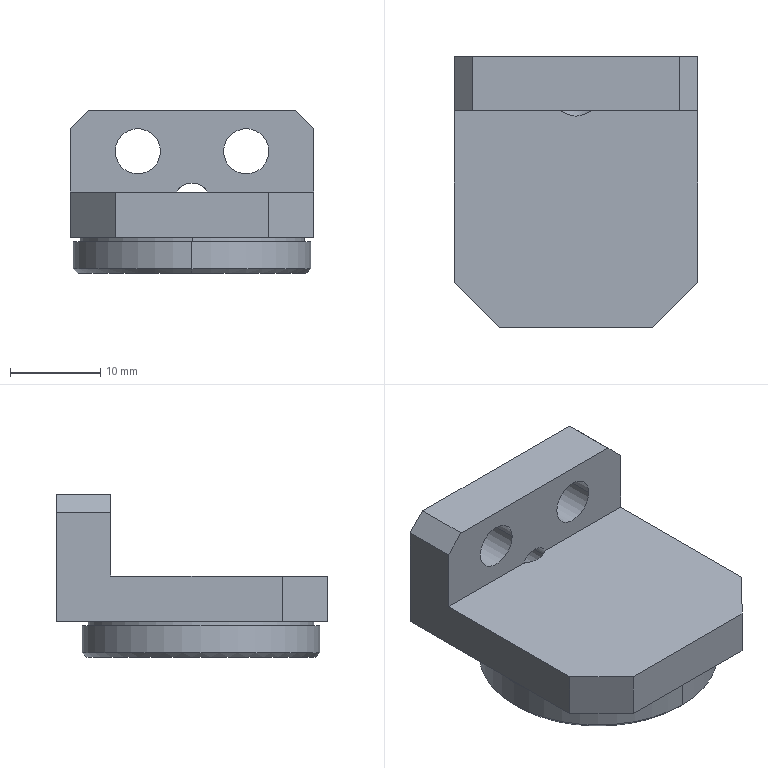NC program | NX | posted with a generic post | part box 27 x 30 x 18 mm
Whole program:
N10 G17 G21 G94 G90
(DRILLING , TOOL : D6A45)
N12 T07 M6
N14 G54
N16 G17 G0 G90 X0. Y10. B0. C0. S5000 M3
N18 G43 Z30. H7
N20 G94 G81 G98 Z-1. F250. R3.
N22 X-6. Y4.5
N24 X6.
N26 G80
N28 G0 X6. Y4.5 Z30.
N30 M5
(DRILLING_COPY , TOOL : 5.0ZT)
N32 T15 M6
N34 G54
N36 G17 G0 G90 X-6. Y4.5 B0. C0. S5000 M3
N38 G43 Z30. H15
N40 G94 G83 G98 Z-9.002 F250. Q2. R3.
N42 X6.
N44 G80
N46 G0 X6. Y4.5 Z30.
N48 M5
(ZLEVEL_PROFILE_COPY_COPY_1 , TOOL : D3)
N50 T03 M6
N52 G54
N54 G17 G0 G90 X-0.088 Y10.392 B0. C0. S9500 M3
N56 G43 Z30. H3
N58 Z1.
N60 G94 G1 X-0.209 Y10.353 Z0.993 F1000.
N62 X-0.331 Y10.242 Z0.985
N64 X-0.399 Y10.093 Z0.976
N66 X-0.401 Y9.913 Z0.967
N68 X-0.333 Y9.76 Z0.958
N70 X-0.209 Y9.647 Z0.949
N72 X-0.038 Y9.592 Z0.94
N74 X0.156 Y9.621 Z0.929
N76 X0.314 Y9.737 Z0.919
N78 X0.401 Y9.913 Z0.909
N80 X0.399 Y10.093 Z0.899
N82 X0.289 Y10.291 Z0.888
N84 X0.09 Y10.4 Z0.876
N86 X-0.063 Z0.868
N88 X-0.209 Y10.353 Z0.86
N90 X-0.331 Y10.242 Z0.851
N92 X-0.399 Y10.093 Z0.842
N94 X-0.401 Y9.913 Z0.833
N96 X-0.333 Y9.76 Z0.824
N98 X-0.209 Y9.647 Z0.815
N100 X-0.038 Y9.592 Z0.806
N102 X0.156 Y9.621 Z0.796
N104 X0.314 Y9.737 Z0.785
N106 X0.401 Y9.913 Z0.775
N108 X0.399 Y10.093 Z0.766
N110 X0.289 Y10.291 Z0.754
N112 X0.09 Y10.4 Z0.742
N114 X-0.063 Z0.734
N116 X-0.209 Y10.353 Z0.726
N118 X-0.331 Y10.242 Z0.717
N120 X-0.399 Y10.093 Z0.709
N122 X-0.401 Y9.913 Z0.699
N124 X-0.333 Y9.76 Z0.69
N126 X-0.209 Y9.647 Z0.682
N128 X-0.038 Y9.592 Z0.672
N130 X0.156 Y9.621 Z0.662
N132 X0.314 Y9.737 Z0.652
N134 X0.401 Y9.913 Z0.641
N136 X0.399 Y10.093 Z0.632
N138 X0.289 Y10.291 Z0.62
N140 X0.09 Y10.4 Z0.608
N142 X-0.063 Z0.6
N144 X-0.209 Y10.353 Z0.592
N146 X-0.331 Y10.242 Z0.583
N148 X-0.399 Y10.093 Z0.575
N150 X-0.401 Y9.913 Z0.565
N152 X-0.333 Y9.76 Z0.557
N154 X-0.209 Y9.647 Z0.548
N156 X-0.038 Y9.592 Z0.539
N158 X0.156 Y9.621 Z0.528
N160 X0.314 Y9.737 Z0.518
N162 X0.401 Y9.913 Z0.508
N164 X0.399 Y10.093 Z0.498
N166 X0.289 Y10.291 Z0.486
N168 X0.09 Y10.4 Z0.474
N170 X-0.063 Z0.466
N172 X-0.209 Y10.353 Z0.458
N174 X-0.331 Y10.242 Z0.45
N176 X-0.399 Y10.093 Z0.441
N178 X-0.401 Y9.913 Z0.432
N180 X-0.333 Y9.76 Z0.423
N182 X-0.209 Y9.647 Z0.414
N184 X-0.038 Y9.592 Z0.405
N186 X0.156 Y9.621 Z0.394
N188 X0.314 Y9.737 Z0.384
N190 X0.401 Y9.913 Z0.374
N192 X0.399 Y10.093 Z0.365
N194 X0.289 Y10.291 Z0.353
N196 X0.09 Y10.4 Z0.341
N198 X-0.063 Z0.333
N200 X-0.209 Y10.353 Z0.325
N202 X-0.331 Y10.242 Z0.316
N204 X-0.399 Y10.093 Z0.307
N206 X-0.401 Y9.913 Z0.298
N208 X-0.333 Y9.76 Z0.289
N210 X-0.209 Y9.647 Z0.28
N212 X-0.038 Y9.592 Z0.271
N214 X0.156 Y9.621 Z0.261
N216 X0.314 Y9.737 Z0.25
N218 X0.401 Y9.913 Z0.24
N220 X0.399 Y10.093 Z0.231
N222 X0.289 Y10.291 Z0.219
N224 X0.09 Y10.4 Z0.207
N226 X-0.063 Z0.199
N228 X-0.209 Y10.353 Z0.191
N230 X-0.331 Y10.242 Z0.182
N232 X-0.399 Y10.093 Z0.174
N234 X-0.401 Y9.913 Z0.164
N236 X-0.333 Y9.76 Z0.156
N238 X-0.209 Y9.647 Z0.147
N240 X-0.038 Y9.592 Z0.137
N242 X0.156 Y9.621 Z0.127
N244 X0.314 Y9.737 Z0.117
N246 X0.401 Y9.913 Z0.106
N248 X0.399 Y10.093 Z0.097
N250 X0.289 Y10.291 Z0.085
N252 X0.09 Y10.4 Z0.073
N254 X-0.063 Z0.065
N256 X-0.209 Y10.353 Z0.057
N258 X-0.331 Y10.242 Z0.049
N260 X-0.399 Y10.093 Z0.04
N262 X-0.401 Y9.913 Z0.031
N264 X-0.333 Y9.76 Z0.022
N266 X-0.209 Y9.647 Z0.013
N268 X-0.038 Y9.592 Z0.004
N270 X0.156 Y9.621 Z-0.007
N272 X0.314 Y9.737 Z-0.017
N274 X0.401 Y9.913 Z-0.027
N276 X0.399 Y10.093 Z-0.037
N278 X0.289 Y10.291 Z-0.049
N280 X0.09 Y10.4 Z-0.06
N282 X-0.063 Z-0.069
N284 X-0.209 Y10.353 Z-0.077
N286 X-0.331 Y10.242 Z-0.085
N288 X-0.399 Y10.093 Z-0.094
N290 X-0.401 Y9.913 Z-0.103
N292 X-0.333 Y9.76 Z-0.112
N294 X-0.209 Y9.647 Z-0.121
N296 X-0.038 Y9.592 Z-0.13
N298 X0.156 Y9.621 Z-0.14
N300 X0.314 Y9.737 Z-0.151
N302 X0.401 Y9.913 Z-0.161
N304 X0.399 Y10.093 Z-0.17
N306 X0.289 Y10.291 Z-0.182
N308 X0.09 Y10.4 Z-0.194
N310 X0. Z-0.199
N312 G3 X-0.4 Y10. R0.4 F1200.
N314 X0. Y10.4 R-0.4
N316 G1 X-0.095 Y10.379 Z-0.209
N318 X-0.141 Y10.365 Z-0.214
N320 X-0.167 Y10.354 Z-0.218
N322 X-0.218 Y10.326 Z-0.224
N324 X-0.288 Y10.265 Z-0.234
N326 X-0.317 Y10.23 Z-0.239
N328 X-0.334 Y10.204 Z-0.242
N330 X-0.362 Y10.15 Z-0.249
N332 X-0.387 Y10.06 Z-0.259
N334 X-0.391 Y10.014 Z-0.264
N336 Y9.984 Z-0.267
N338 X-0.385 Y9.924 Z-0.274
N340 X-0.355 Y9.835 Z-0.283
N342 X-0.333 Y9.795 Z-0.288
N344 X-0.316 Y9.77 Z-0.292
N346 X-0.277 Y9.723 Z-0.298
N348 X-0.203 Y9.666 Z-0.308
N350 X-0.163 Y9.644 Z-0.313
N352 X-0.135 Y9.633 Z-0.317
N354 X-0.076 Y9.616 Z-0.323
N356 X0.017 Y9.609 Z-0.333
N358 X0.062 Y9.614 Z-0.338
N360 X0.092 Y9.62 Z-0.341
N362 X0.15 Y9.638 Z-0.348
N364 X0.229 Y9.683 Z-0.358
N366 X0.287 Y9.732 Z-0.366
N368 X0.326 Y9.782 Z-0.373
N370 X0.354 Y9.834 Z-0.379
N372 X0.374 Y9.888 Z-0.385
N374 X0.387 Y9.944 Z-0.392
N376 X0.4 Y10. Z-0.398
N378 Y10.003
N380 G3 X0. Y10.4 R0.4
N382 G1 X-0.095 Y10.379 Z-0.408
N384 X-0.141 Y10.365 Z-0.413
N386 X-0.167 Y10.354 Z-0.416
N388 X-0.218 Y10.326 Z-0.423
N390 X-0.288 Y10.265 Z-0.433
N392 X-0.317 Y10.23 Z-0.438
N394 X-0.334 Y10.204 Z-0.441
N396 X-0.362 Y10.15 Z-0.448
N398 X-0.387 Y10.06 Z-0.457
N400 X-0.391 Y10.014 Z-0.462
N402 Y9.984 Z-0.466
N404 X-0.384 Y9.924 Z-0.472
N406 X-0.355 Y9.835 Z-0.482
N408 X-0.333 Y9.795 Z-0.487
N410 X-0.316 Y9.77 Z-0.491
N412 X-0.277 Y9.723 Z-0.497
N414 X-0.203 Y9.666 Z-0.507
N416 X-0.163 Y9.645 Z-0.512
N418 X-0.135 Y9.633 Z-0.516
N420 X-0.076 Y9.616 Z-0.522
N422 X0.017 Y9.61 Z-0.532
N424 X0.062 Y9.614 Z-0.537
N426 X0.092 Y9.62 Z-0.54
N428 X0.15 Y9.638 Z-0.547
N430 X0.229 Y9.683 Z-0.557
N432 X0.287 Y9.732 Z-0.565
N434 X0.326 Y9.782 Z-0.572
N436 X0.354 Y9.834 Z-0.578
N438 X0.374 Y9.888 Z-0.584
N440 X0.387 Y9.944 Z-0.591
N442 X0.4 Y10. Z-0.597
N444 Y10.003
N446 G3 X0. Y10.4 R0.4
N448 G1 X-0.095 Y10.379 Z-0.607
N450 X-0.141 Y10.365 Z-0.612
N452 X-0.167 Y10.354 Z-0.615
N454 X-0.218 Y10.326 Z-0.622
N456 X-0.288 Y10.265 Z-0.632
N458 X-0.317 Y10.23 Z-0.636
N460 X-0.334 Y10.204 Z-0.64
N462 X-0.362 Y10.15 Z-0.646
N464 X-0.387 Y10.06 Z-0.656
N466 X-0.391 Y10.014 Z-0.661
N468 Y9.984 Z-0.665
N470 X-0.384 Y9.924 Z-0.671
N472 X-0.355 Y9.835 Z-0.681
N474 X-0.333 Y9.795 Z-0.686
N476 X-0.316 Y9.77 Z-0.69
N478 X-0.277 Y9.723 Z-0.696
N480 X-0.203 Y9.666 Z-0.706
N482 X-0.163 Y9.645 Z-0.711
N484 X-0.135 Y9.633 Z-0.714
N486 X-0.076 Y9.616 Z-0.721
N488 X0.017 Y9.61 Z-0.731
N490 X0.062 Y9.614 Z-0.736
N492 X0.092 Y9.62 Z-0.739
N494 X0.15 Y9.638 Z-0.746
N496 X0.229 Y9.683 Z-0.756
N498 X0.287 Y9.732 Z-0.764
N500 X0.326 Y9.782 Z-0.771
N502 X0.354 Y9.834 Z-0.777
N504 X0.374 Y9.888 Z-0.783
N506 X0.387 Y9.944 Z-0.789
N508 X0.4 Y10. Z-0.796
N510 Y10.003
N512 G3 X0. Y10.4 R0.4
N514 G1 X-0.095 Y10.379 Z-0.806
N516 X-0.141 Y10.365 Z-0.811
N518 X-0.167 Y10.354 Z-0.814
N520 X-0.218 Y10.326 Z-0.821
N522 X-0.288 Y10.265 Z-0.83
N524 X-0.317 Y10.23 Z-0.835
N526 X-0.334 Y10.204 Z-0.839
N528 X-0.362 Y10.15 Z-0.845
N530 X-0.387 Y10.06 Z-0.855
N532 X-0.391 Y10.014 Z-0.86
N534 Y9.984 Z-0.864
N536 X-0.384 Y9.924 Z-0.87
N538 X-0.355 Y9.835 Z-0.88
N540 X-0.333 Y9.795 Z-0.885
N542 X-0.316 Y9.77 Z-0.888
N544 X-0.277 Y9.723 Z-0.895
N546 X-0.203 Y9.666 Z-0.905
N548 X-0.163 Y9.645 Z-0.91
N550 X-0.135 Y9.633 Z-0.913
N552 X-0.076 Y9.616 Z-0.92
N554 X0.017 Y9.61 Z-0.93
N556 X0.062 Y9.614 Z-0.935
N558 X0.092 Y9.62 Z-0.938
N560 X0.15 Y9.638 Z-0.945
N562 X0.229 Y9.683 Z-0.955
N564 X0.287 Y9.732 Z-0.963
N566 X0.326 Y9.782 Z-0.97
N568 X0.354 Y9.834 Z-0.976
N570 X0.374 Y9.888 Z-0.982
N572 X0.387 Y9.944 Z-0.988
N574 X0.4 Y10. Z-0.995
N576 Y10.003
N578 G3 X0. Y10.4 R0.4
N580 G1 X-0.095 Y10.379 Z-1.005
N582 X-0.141 Y10.365 Z-1.01
N584 X-0.167 Y10.354 Z-1.013
N586 X-0.218 Y10.326 Z-1.019
N588 X-0.288 Y10.265 Z-1.029
N590 X-0.317 Y10.23 Z-1.034
N592 X-0.334 Y10.204 Z-1.038
N594 X-0.362 Y10.15 Z-1.044
N596 X-0.387 Y10.06 Z-1.054
N598 X-0.391 Y10.014 Z-1.059
N600 Y9.984 Z-1.063
N602 X-0.384 Y9.924 Z-1.069
N604 X-0.354 Y9.835 Z-1.079
N606 X-0.333 Y9.795 Z-1.084
N608 X-0.316 Y9.77 Z-1.087
N610 X-0.277 Y9.723 Z-1.094
N612 X-0.203 Y9.666 Z-1.104
N614 X-0.163 Y9.645 Z-1.109
N616 X-0.135 Y9.633 Z-1.112
N618 X-0.076 Y9.616 Z-1.119
N620 X0.017 Y9.61 Z-1.129
N622 X0.062 Y9.614 Z-1.134
N624 X0.092 Y9.62 Z-1.137
N626 X0.15 Y9.638 Z-1.144
N628 X0.229 Y9.683 Z-1.153
N630 X0.286 Y9.732 Z-1.162
N632 X0.326 Y9.782 Z-1.169
N634 X0.354 Y9.834 Z-1.175
N636 X0.374 Y9.888 Z-1.181
N638 X0.387 Y9.944 Z-1.187
N640 X0.4 Y10. Z-1.194
N642 Y10.003
N644 G3 X0. Y10.4 R0.4
N646 G1 X-0.095 Y10.379 Z-1.204
N648 X-0.141 Y10.365 Z-1.209
N650 X-0.167 Y10.354 Z-1.212
N652 X-0.218 Y10.326 Z-1.218
N654 X-0.288 Y10.265 Z-1.228
N656 X-0.317 Y10.23 Z-1.233
N658 X-0.334 Y10.204 Z-1.237
N660 X-0.362 Y10.15 Z-1.243
N662 X-0.386 Y10.06 Z-1.253
N664 X-0.391 Y10.014 Z-1.258
N666 Y9.984 Z-1.261
N668 X-0.384 Y9.924 Z-1.268
N670 X-0.354 Y9.835 Z-1.278
N672 X-0.333 Y9.795 Z-1.283
N674 X-0.316 Y9.77 Z-1.286
N676 X-0.277 Y9.723 Z-1.293
N678 X-0.203 Y9.666 Z-1.303
N680 X-0.163 Y9.645 Z-1.308
N682 X-0.135 Y9.633 Z-1.311
N684 X-0.076 Y9.616 Z-1.318
N686 X0.016 Y9.61 Z-1.328
N688 X0.062 Y9.614 Z-1.333
N690 X0.091 Y9.62 Z-1.336
N692 X0.15 Y9.638 Z-1.343
N694 X0.229 Y9.683 Z-1.352
N696 X0.286 Y9.732 Z-1.361
N698 X0.326 Y9.782 Z-1.368
N700 X0.354 Y9.834 Z-1.374
N702 X0.374 Y9.888 Z-1.38
N704 X0.387 Y9.944 Z-1.386
N706 X0.4 Y10. Z-1.392
N708 Y10.003
N710 G3 X0. Y10.4 R0.4
N712 G1 X-0.095 Y10.379 Z-1.403
N714 X-0.141 Y10.365 Z-1.408
N716 X-0.167 Y10.353 Z-1.411
N718 X-0.218 Y10.326 Z-1.417
N720 X-0.288 Y10.265 Z-1.427
N722 X-0.317 Y10.23 Z-1.432
N724 X-0.334 Y10.204 Z-1.435
N726 X-0.362 Y10.15 Z-1.442
N728 X-0.386 Y10.06 Z-1.452
N730 X-0.391 Y10.014 Z-1.457
N732 Y9.984 Z-1.46
N734 X-0.384 Y9.924 Z-1.467
N736 X-0.354 Y9.835 Z-1.477
N738 X-0.333 Y9.796 Z-1.482
N740 X-0.316 Y9.77 Z-1.485
N742 X-0.277 Y9.723 Z-1.492
N744 X-0.203 Y9.667 Z-1.502
N746 X-0.163 Y9.645 Z-1.507
N748 X-0.135 Y9.633 Z-1.51
N750 X-0.076 Y9.616 Z-1.517
N752 X0.016 Y9.61 Z-1.527
N754 X0.061 Y9.614 Z-1.532
N756 X0.091 Y9.62 Z-1.535
N758 X0.15 Y9.638 Z-1.542
N760 X0.228 Y9.683 Z-1.551
N762 X0.264 Y9.71 Z-1.556
N764 X0.286 Y9.732 Z-1.56
N766 X0.326 Y9.782 Z-1.566
N768 X0.354 Y9.834 Z-1.573
N770 X0.374 Y9.888 Z-1.579
N772 X0.387 Y9.944 Z-1.585
N774 X0.4 Y10. Z-1.591
N776 Y10.003
N778 G3 X0. Y10.4 R0.4
N780 G1 X-0.095 Y10.379 Z-1.602
N782 X-0.14 Y10.365 Z-1.607
N784 X-0.167 Y10.353 Z-1.61
N786 X-0.218 Y10.326 Z-1.616
N788 X-0.288 Y10.265 Z-1.626
N790 X-0.317 Y10.23 Z-1.631
N792 X-0.334 Y10.204 Z-1.634
N794 X-0.362 Y10.15 Z-1.641
N796 X-0.386 Y10.06 Z-1.651
N798 X-0.391 Y10.015 Z-1.656
N800 Y9.984 Z-1.659
N802 X-0.384 Y9.924 Z-1.666
N804 X-0.354 Y9.835 Z-1.676
N806 X-0.333 Y9.796 Z-1.681
N808 X-0.316 Y9.77 Z-1.684
N810 X-0.277 Y9.723 Z-1.691
N812 X-0.204 Y9.665 Z-1.701
N814 X-0.164 Y9.644 Z-1.706
N816 X-0.135 Y9.634 Z-1.709
N818 X-0.076 Y9.616 Z-1.716
N820 X0.016 Y9.61 Z-1.726
N822 X0.061 Y9.614 Z-1.73
N824 X0.091 Y9.62 Z-1.734
N826 X0.15 Y9.638 Z-1.741
N828 X0.23 Y9.682 Z-1.75
N830 X0.264 Y9.71 Z-1.755
N832 X0.286 Y9.732 Z-1.758
N834 X0.325 Y9.783 Z-1.765
N836 X0.354 Y9.834 Z-1.772
N838 X0.374 Y9.888 Z-1.778
N840 X0.387 Y9.944 Z-1.784
N842 X0.4 Y10. Z-1.79
N844 Y10.003
N846 G3 X0. Y10.4 R0.4
N848 G1 X-0.095 Y10.379 Z-1.801
N850 X-0.14 Y10.365 Z-1.806
N852 X-0.167 Y10.353 Z-1.809
N854 X-0.218 Y10.326 Z-1.815
N856 X-0.288 Y10.265 Z-1.825
N858 X-0.316 Y10.23 Z-1.83
N860 X-0.334 Y10.204 Z-1.833
N862 X-0.362 Y10.15 Z-1.84
N864 X-0.386 Y10.06 Z-1.85
N866 X-0.391 Y10.015 Z-1.855
N868 Y9.984 Z-1.858
N870 X-0.384 Y9.924 Z-1.865
N872 X-0.354 Y9.835 Z-1.875
N874 X-0.333 Y9.796 Z-1.88
N876 X-0.316 Y9.77 Z-1.883
N878 X-0.277 Y9.723 Z-1.89
N880 X-0.204 Y9.665 Z-1.9
N882 X-0.164 Y9.644 Z-1.905
N884 X-0.135 Y9.634 Z-1.908
N886 X-0.076 Y9.616 Z-1.915
N888 X0.017 Y9.608 Z-1.924
N890 X0.061 Y9.613 Z-1.929
N892 X0.091 Y9.62 Z-1.933
N894 X0.15 Y9.638 Z-1.939
N896 X0.229 Y9.682 Z-1.949
N898 X0.263 Y9.71 Z-1.954
N900 X0.286 Y9.732 Z-1.957
N902 X0.325 Y9.783 Z-1.964
N904 X0.354 Y9.834 Z-1.971
N906 X0.374 Y9.888 Z-1.977
N908 X0.387 Y9.944 Z-1.983
N910 X0.4 Y10. Z-1.989
N912 Y10.003
N914 G3 X0. Y10.4 R0.4
N916 G1 X-0.095 Y10.379 Z-1.999
N918 X-0.14 Y10.365 Z-2.005
N920 X-0.167 Y10.353 Z-2.008
N922 X-0.218 Y10.326 Z-2.014
N924 X-0.288 Y10.265 Z-2.024
N926 X-0.316 Y10.23 Z-2.029
N928 X-0.333 Y10.204 Z-2.032
N930 X-0.362 Y10.15 Z-2.039
N932 X-0.386 Y10.06 Z-2.049
N934 X-0.391 Y10.015 Z-2.054
N936 Y9.984 Z-2.057
N938 X-0.384 Y9.924 Z-2.064
N940 X-0.354 Y9.836 Z-2.074
N942 X-0.333 Y9.796 Z-2.079
N944 X-0.316 Y9.77 Z-2.082
N946 X-0.277 Y9.723 Z-2.089
N948 X-0.204 Y9.665 Z-2.099
N950 X-0.164 Y9.644 Z-2.103
N952 X-0.136 Y9.632 Z-2.107
N954 X-0.076 Y9.616 Z-2.114
N956 X0.019 Y9.609 Z-2.124
N958 X0.065 Y9.613 Z-2.129
N960 X0.15 Y9.638 Z-2.138
N962 X0.23 Y9.682 Z-2.148
N964 X0.264 Y9.711 Z-2.153
N966 X0.286 Y9.733 Z-2.156
N968 X0.325 Y9.783 Z-2.163
N970 X0.354 Y9.834 Z-2.169
N972 X0.374 Y9.888 Z-2.176
N974 X0.387 Y9.944 Z-2.182
N976 X0.4 Y10. Z-2.188
N978 Y10.003
N980 G3 X0. Y10.4 R0.4
N982 G1 X-0.095 Y10.379 Z-2.198
N984 X-0.14 Y10.365 Z-2.204
N986 X-0.167 Y10.353 Z-2.207
N988 X-0.218 Y10.326 Z-2.213
N990 X-0.288 Y10.265 Z-2.223
N992 X-0.316 Y10.23 Z-2.228
N994 X-0.333 Y10.204 Z-2.231
N996 X-0.362 Y10.15 Z-2.238
N998 X-0.386 Y10.06 Z-2.248
N1000 X-0.391 Y10.015 Z-2.253
N1002 Y9.984 Z-2.256
N1004 X-0.384 Y9.924 Z-2.263
N1006 X-0.354 Y9.836 Z-2.273
N1008 X-0.333 Y9.796 Z-2.278
N1010 X-0.316 Y9.771 Z-2.281
N1012 X-0.277 Y9.723 Z-2.288
N1014 X-0.204 Y9.665 Z-2.297
N1016 X-0.164 Y9.644 Z-2.302
N1018 X-0.136 Y9.632 Z-2.306
N1020 X-0.076 Y9.616 Z-2.312
N1022 X0.019 Y9.609 Z-2.323
N1024 X0.065 Y9.613 Z-2.328
N1026 X0.15 Y9.638 Z-2.337
N1028 X0.229 Y9.682 Z-2.347
N1030 X0.264 Y9.71 Z-2.352
N1032 X0.286 Y9.733 Z-2.355
N1034 X0.325 Y9.783 Z-2.362
N1036 X0.354 Y9.834 Z-2.368
N1038 X0.374 Y9.888 Z-2.375
N1040 X0.387 Y9.944 Z-2.381
N1042 X0.4 Y10. Z-2.387
N1044 Y10.003
N1046 G3 X0. Y10.4 R0.4
N1048 G1 X-0.094 Y10.379 Z-2.397
N1050 X-0.14 Y10.365 Z-2.402
N1052 X-0.167 Y10.353 Z-2.406
N1054 X-0.218 Y10.326 Z-2.412
N1056 X-0.288 Y10.265 Z-2.422
N1058 X-0.316 Y10.23 Z-2.427
N1060 X-0.333 Y10.204 Z-2.43
N1062 X-0.362 Y10.15 Z-2.437
N1064 X-0.386 Y10.06 Z-2.447
N1066 X-0.391 Y10.015 Z-2.452
N1068 Y9.984 Z-2.455
N1070 X-0.384 Y9.924 Z-2.462
N1072 X-0.354 Y9.836 Z-2.471
N1074 X-0.317 Y9.77 Z-2.48
N1076 X-0.277 Y9.723 Z-2.486
N1078 X-0.201 Y9.664 Z-2.497
N1080 X-0.161 Y9.643 Z-2.502
N1082 X-0.076 Y9.616 Z-2.511
N1084 X0.017 Y9.609 Z-2.521
N1086 X0.062 Y9.613 Z-2.526
N1088 X0.092 Y9.619 Z-2.53
N1090 X0.15 Y9.638 Z-2.536
N1092 X0.231 Y9.684 Z-2.546
N1094 X0.266 Y9.713 Z-2.551
N1096 X0.287 Y9.734 Z-2.554
N1098 X0.325 Y9.783 Z-2.561
N1100 X0.354 Y9.834 Z-2.567
N1102 X0.374 Y9.888 Z-2.574
N1104 X0.387 Y9.944 Z-2.58
N1106 X0.4 Y10. Z-2.586
N1108 Y10.003
N1110 G3 X0. Y10.4 R0.4
N1112 G1 X-0.094 Y10.379 Z-2.596
N1114 X-0.14 Y10.365 Z-2.601
N1116 X-0.167 Y10.353 Z-2.605
N1118 X-0.218 Y10.326 Z-2.611
N1120 X-0.288 Y10.265 Z-2.621
N1122 X-0.316 Y10.23 Z-2.626
N1124 X-0.333 Y10.204 Z-2.629
N1126 X-0.362 Y10.15 Z-2.636
N1128 X-0.386 Y10.06 Z-2.646
N1130 X-0.391 Y10.015 Z-2.651
N1132 Y9.984 Z-2.654
N1134 X-0.384 Y9.924 Z-2.661
N1136 X-0.354 Y9.836 Z-2.67
N1138 X-0.334 Y9.795 Z-2.675
N1140 X-0.317 Y9.77 Z-2.679
N1142 X-0.277 Y9.723 Z-2.685
N1144 X-0.201 Y9.665 Z-2.695
N1146 X-0.161 Y9.643 Z-2.701
N1148 X-0.076 Y9.616 Z-2.71
N1150 X0.017 Y9.609 Z-2.72
N1152 X0.062 Y9.613 Z-2.725
N1154 X0.091 Y9.619 Z-2.728
N1156 X0.15 Y9.639 Z-2.735
N1158 X0.231 Y9.684 Z-2.745
N1160 X0.266 Y9.713 Z-2.75
N1162 X0.287 Y9.734 Z-2.753
N1164 X0.325 Y9.783 Z-2.76
N1166 X0.354 Y9.834 Z-2.766
N1168 X0.374 Y9.888 Z-2.772
N1170 X0.387 Y9.944 Z-2.779
N1172 X0.4 Y10. Z-2.785
N1174 Y10.003
N1176 G3 X0. Y10.4 R0.4
N1178 G1 X-0.094 Y10.379 Z-2.795
N1180 X-0.14 Y10.365 Z-2.8
N1182 X-0.167 Y10.353 Z-2.803
N1184 X-0.218 Y10.326 Z-2.81
N1186 X-0.288 Y10.265 Z-2.82
N1188 X-0.316 Y10.23 Z-2.825
N1190 X-0.333 Y10.204 Z-2.828
N1192 X-0.362 Y10.15 Z-2.835
N1194 X-0.386 Y10.06 Z-2.844
N1196 X-0.391 Y10.015 Z-2.849
N1198 Y9.984 Z-2.853
N1200 X-0.384 Y9.924 Z-2.859
N1202 X-0.354 Y9.836 Z-2.869
N1204 X-0.334 Y9.795 Z-2.874
N1206 X-0.317 Y9.77 Z-2.878
N1208 X-0.277 Y9.723 Z-2.884
N1210 X-0.202 Y9.665 Z-2.894
N1212 X-0.161 Y9.643 Z-2.899
N1214 X-0.076 Y9.616 Z-2.909
N1216 X0.017 Y9.609 Z-2.919
N1218 X0.061 Y9.613 Z-2.924
N1220 X0.091 Y9.619 Z-2.927
N1222 X0.15 Y9.639 Z-2.934
N1224 X0.231 Y9.684 Z-2.944
N1226 X0.265 Y9.712 Z-2.949
N1228 X0.287 Y9.734 Z-2.952
N1230 X0.325 Y9.783 Z-2.959
N1232 X0.354 Y9.834 Z-2.965
N1234 X0.374 Y9.888 Z-2.971
N1236 X0.387 Y9.944 Z-2.978
N1238 X0.4 Y10. Z-2.984
N1240 Y10.003
N1242 G3 X0. Y10.4 R0.4
N1244 G1 X-0.094 Y10.379 Z-2.994
N1246 X-0.14 Y10.365 Z-2.999
N1248 X-0.167 Y10.353 Z-3.002
N1250 X-0.218 Y10.326 Z-3.009
N1252 X-0.287 Y10.265 Z-3.018
N1254 X-0.316 Y10.23 Z-3.023
N1256 X-0.333 Y10.204 Z-3.027
N1258 X-0.362 Y10.15 Z-3.034
N1260 X-0.386 Y10.06 Z-3.043
N1262 X-0.39 Y10.015 Z-3.048
N1264 X-0.391 Y9.984 Z-3.052
N1266 X-0.384 Y9.924 Z-3.058
N1268 X-0.354 Y9.836 Z-3.068
N1270 X-0.334 Y9.796 Z-3.073
N1272 X-0.317 Y9.77 Z-3.077
N1274 X-0.277 Y9.723 Z-3.083
N1276 X-0.202 Y9.665 Z-3.093
N1278 X-0.161 Y9.643 Z-3.098
N1280 X-0.134 Y9.632 Z-3.102
N1282 X-0.076 Y9.616 Z-3.108
N1284 X0.019 Y9.609 Z-3.118
N1286 X0.065 Y9.614 Z-3.123
N1288 X0.15 Y9.639 Z-3.133
N1290 X0.229 Y9.683 Z-3.143
N1292 X0.263 Y9.71 Z-3.147
N1294 X0.285 Y9.733 Z-3.151
N1296 X0.325 Y9.783 Z-3.158
N1298 X0.354 Y9.834 Z-3.164
N1300 X0.374 Y9.888 Z-3.17
N1302 X0.387 Y9.944 Z-3.176
N1304 X0.4 Y10. Z-3.183
N1306 Y10.003
N1308 G3 X0. Y10.4 R0.4
N1310 G1 X-0.094 Y10.379 Z-3.193
N1312 X-0.14 Y10.365 Z-3.198
N1314 X-0.167 Y10.353 Z-3.201
N1316 X-0.218 Y10.326 Z-3.208
N1318 X-0.287 Y10.265 Z-3.217
N1320 X-0.316 Y10.23 Z-3.222
N1322 X-0.333 Y10.204 Z-3.226
N1324 X-0.362 Y10.15 Z-3.232
N1326 X-0.386 Y10.06 Z-3.242
N1328 X-0.39 Y10.015 Z-3.247
N1330 X-0.391 Y9.985 Z-3.251
N1332 X-0.384 Y9.924 Z-3.257
N1334 X-0.355 Y9.835 Z-3.267
N1336 X-0.334 Y9.796 Z-3.272
N1338 X-0.317 Y9.77 Z-3.275
N1340 X-0.277 Y9.723 Z-3.282
N1342 X-0.202 Y9.665 Z-3.292
N1344 X-0.161 Y9.643 Z-3.297
N1346 X-0.134 Y9.632 Z-3.301
N1348 X-0.076 Y9.616 Z-3.307
N1350 X0.019 Y9.609 Z-3.317
N1352 X0.065 Y9.614 Z-3.322
N1354 X0.094 Y9.62 Z-3.325
N1356 X0.15 Y9.639 Z-3.332
N1358 X0.231 Y9.684 Z-3.342
N1360 X0.266 Y9.713 Z-3.347
N1362 X0.287 Y9.735 Z-3.35
N1364 X0.325 Y9.783 Z-3.357
N1366 X0.354 Y9.834 Z-3.363
N1368 X0.374 Y9.888 Z-3.369
N1370 X0.387 Y9.944 Z-3.375
N1372 X0.4 Y10. Z-3.382
N1374 Y10.003
N1376 G3 X0. Y10.4 R0.4
N1378 G1 X-0.094 Y10.379 Z-3.392
N1380 X-0.14 Y10.365 Z-3.397
N1382 X-0.166 Y10.353 Z-3.4
N1384 X-0.218 Y10.326 Z-3.406
N1386 X-0.287 Y10.265 Z-3.416
N1388 X-0.316 Y10.23 Z-3.421
N1390 X-0.333 Y10.204 Z-3.425
N1392 X-0.362 Y10.15 Z-3.431
N1394 X-0.386 Y10.06 Z-3.441
N1396 X-0.39 Y10.015 Z-3.446
N1398 X-0.391 Y9.985 Z-3.45
N1400 X-0.384 Y9.924 Z-3.456
N1402 X-0.355 Y9.836 Z-3.466
N1404 X-0.334 Y9.796 Z-3.471
N1406 X-0.317 Y9.77 Z-3.474
N1408 X-0.277 Y9.723 Z-3.481
N1410 X-0.202 Y9.665 Z-3.491
N1412 X-0.161 Y9.643 Z-3.496
N1414 X-0.134 Y9.632 Z-3.499
N1416 X-0.076 Y9.616 Z-3.506
N1418 X0.019 Y9.61 Z-3.516
N1420 X0.065 Y9.614 Z-3.521
N1422 X0.094 Y9.62 Z-3.524
N1424 X0.15 Y9.639 Z-3.531
N1426 X0.231 Y9.684 Z-3.541
N1428 X0.266 Y9.713 Z-3.546
N1430 X0.287 Y9.735 Z-3.549
N1432 X0.325 Y9.783 Z-3.556
N1434 X0.354 Y9.834 Z-3.562
N1436 X0.374 Y9.888 Z-3.568
N1438 X0.387 Y9.944 Z-3.574
N1440 X0.4 Y10. Z-3.581
N1442 Y10.003
N1444 G3 X0. Y10.4 R0.4
N1446 G1 X-0.094 Y10.379 Z-3.591
N1448 X-0.14 Y10.365 Z-3.596
N1450 X-0.166 Y10.353 Z-3.599
N1452 X-0.218 Y10.326 Z-3.605
N1454 X-0.287 Y10.265 Z-3.615
N1456 X-0.316 Y10.23 Z-3.62
N1458 X-0.333 Y10.204 Z-3.624
N1460 X-0.362 Y10.15 Z-3.63
N1462 X-0.386 Y10.06 Z-3.64
N1464 X-0.39 Y10.015 Z-3.645
N1466 Y9.985 Z-3.648
N1468 X-0.384 Y9.924 Z-3.655
N1470 X-0.355 Y9.836 Z-3.665
N1472 X-0.334 Y9.796 Z-3.67
N1474 X-0.317 Y9.77 Z-3.673
N1476 X-0.276 Y9.724 Z-3.68
N1478 X-0.202 Y9.665 Z-3.69
N1480 X-0.161 Y9.643 Z-3.695
N1482 X-0.134 Y9.632 Z-3.698
N1484 X-0.076 Y9.617 Z-3.705
N1486 X0.019 Y9.61 Z-3.715
N1488 X0.065 Y9.614 Z-3.72
N1490 X0.093 Y9.62 Z-3.723
N1492 X0.15 Y9.639 Z-3.73
N1494 X0.231 Y9.684 Z-3.74
N1496 X0.265 Y9.713 Z-3.745
N1498 X0.287 Y9.735 Z-3.748
N1500 X0.325 Y9.783 Z-3.755
N1502 X0.354 Y9.834 Z-3.761
N1504 X0.374 Y9.888 Z-3.767
N1506 X0.387 Y9.944 Z-3.773
N1508 X0.4 Y10. Z-3.779
N1510 Y10.003
N1512 G3 X0. Y10.4 R0.4
N1514 G1 X-0.094 Y10.379 Z-3.79
N1516 X-0.14 Y10.365 Z-3.795
N1518 X-0.166 Y10.353 Z-3.798
N1520 X-0.218 Y10.326 Z-3.804
N1522 X-0.287 Y10.265 Z-3.814
N1524 X-0.316 Y10.23 Z-3.819
N1526 X-0.333 Y10.204 Z-3.822
N1528 X-0.362 Y10.15 Z-3.829
N1530 X-0.386 Y10.06 Z-3.839
N1532 X-0.39 Y10.015 Z-3.844
N1534 Y9.985 Z-3.847
N1536 X-0.384 Y9.924 Z-3.854
N1538 X-0.355 Y9.836 Z-3.864
N1540 X-0.334 Y9.796 Z-3.869
N1542 X-0.317 Y9.77 Z-3.872
N1544 X-0.276 Y9.724 Z-3.879
N1546 X-0.202 Y9.665 Z-3.889
N1548 X-0.161 Y9.644 Z-3.894
N1550 X-0.134 Y9.632 Z-3.897
N1552 X-0.076 Y9.617 Z-3.904
N1554 X0.019 Y9.61 Z-3.914
N1556 X0.064 Y9.614 Z-3.919
N1558 X0.093 Y9.62 Z-3.922
N1560 X0.15 Y9.639 Z-3.929
N1562 X0.23 Y9.684 Z-3.938
N1564 X0.265 Y9.713 Z-3.943
N1566 X0.287 Y9.735 Z-3.947
N1568 X0.325 Y9.783 Z-3.954
N1570 X0.354 Y9.834 Z-3.96
N1572 X0.374 Y9.888 Z-3.966
N1574 X0.387 Y9.944 Z-3.972
N1576 X0.4 Y10. Z-3.978
N1578 Y10.003
N1580 G3 X0. Y10.4 R0.4
N1582 G1 X-0.094 Y10.379 Z-3.989
N1584 X-0.14 Y10.365 Z-3.994
N1586 X-0.167 Y10.354 Z-3.997
N1588 X-0.218 Y10.326 Z-4.003
N1590 X-0.288 Y10.264 Z-4.013
N1592 X-0.317 Y10.228 Z-4.018
N1594 X-0.334 Y10.203 Z-4.021
N1596 X-0.362 Y10.15 Z-4.028
N1598 X-0.386 Y10.06 Z-4.038
N1600 X-0.39 Y10.015 Z-4.043
N1602 Y9.984 Z-4.046
N1604 X-0.384 Y9.924 Z-4.053
N1606 X-0.355 Y9.836 Z-4.063
N1608 X-0.334 Y9.796 Z-4.068
N1610 X-0.317 Y9.771 Z-4.071
N1612 X-0.276 Y9.724 Z-4.078
N1614 X-0.202 Y9.665 Z-4.088
N1616 X-0.161 Y9.644 Z-4.093
N1618 X-0.134 Y9.632 Z-4.096
N1620 X-0.076 Y9.617 Z-4.103
N1622 X0.018 Y9.61 Z-4.113
N1624 X0.064 Y9.614 Z-4.118
N1626 X0.093 Y9.62 Z-4.121
N1628 X0.15 Y9.639 Z-4.128
N1630 X0.23 Y9.684 Z-4.137
N1632 X0.265 Y9.713 Z-4.142
N1634 X0.287 Y9.735 Z-4.146
N1636 X0.325 Y9.783 Z-4.152
N1638 X0.354 Y9.834 Z-4.159
N1640 X0.374 Y9.888 Z-4.165
N1642 X0.387 Y9.944 Z-4.171
N1644 X0.4 Y10. Z-4.177
N1646 Y10.003
N1648 G3 X0. Y10.4 R0.4
N1650 G1 X-0.094 Y10.379 Z-4.188
N1652 X-0.14 Y10.365 Z-4.193
N1654 X-0.167 Y10.354 Z-4.196
N1656 X-0.218 Y10.326 Z-4.202
N1658 X-0.288 Y10.264 Z-4.212
N1660 X-0.317 Y10.228 Z-4.217
N1662 X-0.334 Y10.203 Z-4.22
N1664 X-0.362 Y10.15 Z-4.227
N1666 X-0.386 Y10.06 Z-4.237
N1668 X-0.39 Y10.015 Z-4.242
N1670 Y9.984 Z-4.245
N1672 X-0.384 Y9.924 Z-4.252
N1674 X-0.355 Y9.836 Z-4.262
N1676 X-0.334 Y9.796 Z-4.267
N1678 X-0.317 Y9.771 Z-4.27
N1680 X-0.276 Y9.724 Z-4.277
N1682 X-0.202 Y9.666 Z-4.287
N1684 X-0.161 Y9.644 Z-4.292
N1686 X-0.134 Y9.633 Z-4.295
N1688 X-0.076 Y9.617 Z-4.302
N1690 X0.018 Y9.61 Z-4.312
N1692 X0.064 Y9.614 Z-4.317
N1694 X0.093 Y9.62 Z-4.32
N1696 X0.15 Y9.639 Z-4.326
N1698 X0.23 Y9.684 Z-4.336
N1700 X0.265 Y9.713 Z-4.341
N1702 X0.286 Y9.735 Z-4.345
N1704 X0.325 Y9.783 Z-4.351
N1706 X0.354 Y9.834 Z-4.358
N1708 X0.374 Y9.888 Z-4.364
N1710 X0.387 Y9.944 Z-4.37
N1712 X0.4 Y10. Z-4.376
N1714 Y10.003
N1716 G3 X0. Y10.4 R0.4
N1718 G1 X-0.094 Y10.379 Z-4.386
N1720 X-0.14 Y10.365 Z-4.392
N1722 X-0.167 Y10.354 Z-4.395
N1724 X-0.218 Y10.326 Z-4.401
N1726 X-0.288 Y10.264 Z-4.411
N1728 X-0.317 Y10.228 Z-4.416
N1730 X-0.334 Y10.203 Z-4.419
N1732 X-0.362 Y10.15 Z-4.426
N1734 X-0.386 Y10.06 Z-4.436
N1736 X-0.39 Y10.015 Z-4.441
N1738 Y9.984 Z-4.444
N1740 X-0.384 Y9.924 Z-4.451
N1742 X-0.355 Y9.836 Z-4.461
N1744 X-0.334 Y9.796 Z-4.466
N1746 X-0.317 Y9.771 Z-4.469
N1748 X-0.276 Y9.724 Z-4.476
N1750 X-0.202 Y9.666 Z-4.486
N1752 X-0.161 Y9.644 Z-4.491
N1754 X-0.134 Y9.633 Z-4.494
N1756 X-0.076 Y9.617 Z-4.501
N1758 X0.018 Y9.61 Z-4.511
N1760 X0.064 Y9.614 Z-4.516
N1762 X0.093 Y9.62 Z-4.519
N1764 X0.15 Y9.639 Z-4.525
N1766 X0.23 Y9.684 Z-4.535
N1768 X0.265 Y9.713 Z-4.54
N1770 X0.286 Y9.735 Z-4.544
N1772 X0.325 Y9.783 Z-4.55
N1774 X0.354 Y9.834 Z-4.556
N1776 X0.374 Y9.888 Z-4.563
N1778 X0.387 Y9.944 Z-4.569
N1780 X0.4 Y10. Z-4.575
N1782 Y10.003
N1784 G3 X0. Y10.4 R0.4
N1786 G1 X-0.094 Y10.379 Z-4.585
N1788 X-0.14 Y10.365 Z-4.591
N1790 X-0.167 Y10.354 Z-4.594
N1792 X-0.218 Y10.326 Z-4.6
N1794 X-0.288 Y10.264 Z-4.61
N1796 X-0.317 Y10.228 Z-4.615
N1798 X-0.333 Y10.203 Z-4.618
N1800 X-0.362 Y10.15 Z-4.625
N1802 X-0.386 Y10.06 Z-4.635
N1804 X-0.39 Y10.015 Z-4.64
N1806 Y9.985 Z-4.643
N1808 X-0.384 Y9.924 Z-4.65
N1810 X-0.355 Y9.836 Z-4.66
N1812 X-0.334 Y9.796 Z-4.664
N1814 X-0.317 Y9.771 Z-4.668
N1816 X-0.276 Y9.724 Z-4.675
N1818 X-0.202 Y9.666 Z-4.685
N1820 X-0.161 Y9.644 Z-4.69
N1822 X-0.134 Y9.633 Z-4.693
N1824 X-0.076 Y9.617 Z-4.699
N1826 X0.018 Y9.61 Z-4.709
N1828 X0.064 Y9.614 Z-4.715
N1830 X0.093 Y9.62 Z-4.718
N1832 X0.15 Y9.639 Z-4.724
N1834 X0.23 Y9.684 Z-4.734
N1836 X0.264 Y9.713 Z-4.739
N1838 X0.286 Y9.734 Z-4.742
N1840 X0.325 Y9.783 Z-4.749
N1842 X0.354 Y9.834 Z-4.755
N1844 X0.374 Y9.888 Z-4.762
N1846 X0.387 Y9.944 Z-4.768
N1848 X0.4 Y10. Z-4.774
N1850 Y10.003
N1852 G3 X0. Y10.4 R0.4
N1854 G1 X-0.094 Y10.379 Z-4.784
N1856 X-0.14 Y10.365 Z-4.789
N1858 X-0.167 Y10.354 Z-4.793
N1860 X-0.218 Y10.326 Z-4.799
N1862 X-0.288 Y10.264 Z-4.809
N1864 X-0.317 Y10.229 Z-4.814
N1866 X-0.333 Y10.203 Z-4.817
N1868 X-0.362 Y10.15 Z-4.824
N1870 X-0.386 Y10.06 Z-4.834
N1872 X-0.39 Y10.015 Z-4.839
N1874 Y9.985 Z-4.842
N1876 X-0.384 Y9.924 Z-4.849
N1878 X-0.355 Y9.836 Z-4.858
N1880 X-0.334 Y9.797 Z-4.863
N1882 X-0.317 Y9.771 Z-4.867
N1884 X-0.276 Y9.724 Z-4.874
N1886 X-0.202 Y9.666 Z-4.884
N1888 X-0.161 Y9.644 Z-4.889
N1890 X-0.134 Y9.633 Z-4.892
N1892 X-0.076 Y9.617 Z-4.898
N1894 X0.018 Y9.61 Z-4.908
N1896 X0.064 Y9.615 Z-4.913
N1898 X0.093 Y9.62 Z-4.917
N1900 X0.15 Y9.639 Z-4.923
N1902 X0.23 Y9.684 Z-4.933
N1904 X0.264 Y9.713 Z-4.938
N1906 X0.286 Y9.734 Z-4.941
N1908 X0.325 Y9.783 Z-4.948
N1910 X0.354 Y9.834 Z-4.954
N1912 X0.374 Y9.888 Z-4.961
N1914 X0.386 Y9.944 Z-4.967
N1916 X0.4 Y10. Z-4.973
N1918 Y10.003
N1920 G3 X0. Y10.4 R0.4
N1922 G1 X-0.094 Y10.379 Z-4.983
N1924 X-0.14 Y10.365 Z-4.988
N1926 X-0.167 Y10.354 Z-4.992
N1928 X-0.218 Y10.326 Z-4.998
N1930 X-0.288 Y10.264 Z-5.008
N1932 X-0.317 Y10.229 Z-5.013
N1934 X-0.333 Y10.203 Z-5.016
N1936 X-0.362 Y10.15 Z-5.023
N1938 X-0.386 Y10.06 Z-5.033
N1940 X-0.39 Y10.015 Z-5.038
N1942 Y9.985 Z-5.041
N1944 X-0.384 Y9.924 Z-5.048
N1946 X-0.355 Y9.836 Z-5.057
N1948 X-0.334 Y9.797 Z-5.062
N1950 X-0.317 Y9.771 Z-5.066
N1952 X-0.276 Y9.724 Z-5.072
N1954 X-0.202 Y9.666 Z-5.082
N1956 X-0.162 Y9.644 Z-5.087
N1958 X-0.134 Y9.633 Z-5.091
N1960 X-0.076 Y9.617 Z-5.097
N1962 X0.018 Y9.61 Z-5.107
N1964 X0.063 Y9.615 Z-5.112
N1966 X0.093 Y9.621 Z-5.116
N1968 X0.149 Y9.639 Z-5.122
N1970 X0.229 Y9.684 Z-5.132
N1972 X0.264 Y9.713 Z-5.137
N1974 X0.286 Y9.734 Z-5.14
N1976 X0.325 Y9.783 Z-5.147
N1978 X0.354 Y9.834 Z-5.153
N1980 X0.374 Y9.888 Z-5.159
N1982 X0.386 Y9.944 Z-5.166
N1984 X0.4 Y10. Z-5.172
N1986 Y10.003
N1988 G3 X0. Y10.4 R0.4
N1990 G1 X-0.094 Y10.379 Z-5.182
N1992 X-0.14 Y10.365 Z-5.187
N1994 X-0.167 Y10.354 Z-5.19
N1996 X-0.217 Y10.326 Z-5.197
N1998 X-0.288 Y10.264 Z-5.207
N2000 X-0.317 Y10.229 Z-5.212
N2002 X-0.333 Y10.203 Z-5.215
N2004 X-0.362 Y10.15 Z-5.222
N2006 X-0.386 Y10.06 Z-5.231
N2008 X-0.39 Y10.015 Z-5.236
N2010 Y9.985 Z-5.24
N2012 X-0.384 Y9.924 Z-5.246
N2014 X-0.355 Y9.836 Z-5.256
N2016 X-0.334 Y9.797 Z-5.261
N2018 X-0.317 Y9.771 Z-5.265
N2020 X-0.276 Y9.724 Z-5.271
N2022 X-0.202 Y9.666 Z-5.281
N2024 X-0.162 Y9.645 Z-5.286
N2026 X-0.134 Y9.633 Z-5.29
N2028 X-0.076 Y9.617 Z-5.296
N2030 X0.018 Y9.61 Z-5.306
N2032 X0.063 Y9.615 Z-5.311
N2034 X0.092 Y9.621 Z-5.315
N2036 X0.149 Y9.639 Z-5.321
N2038 X0.229 Y9.684 Z-5.331
N2040 X0.264 Y9.713 Z-5.336
N2042 X0.286 Y9.734 Z-5.339
N2044 X0.325 Y9.783 Z-5.346
N2046 X0.354 Y9.834 Z-5.352
N2048 X0.374 Y9.888 Z-5.358
N2050 X0.386 Y9.944 Z-5.365
N2052 X0.4 Y10. Z-5.371
N2054 Y10.003
N2056 G3 X0. Y10.4 R0.4
N2058 G1 X-0.094 Y10.379 Z-5.381
N2060 X-0.14 Y10.365 Z-5.386
N2062 X-0.166 Y10.354 Z-5.389
N2064 X-0.217 Y10.325 Z-5.396
N2066 X-0.288 Y10.264 Z-5.406
N2068 X-0.317 Y10.229 Z-5.411
N2070 X-0.333 Y10.203 Z-5.414
N2072 X-0.362 Y10.15 Z-5.421
N2074 X-0.386 Y10.06 Z-5.43
N2076 X-0.391 Y10.015 Z-5.435
N2078 X-0.39 Y9.985 Z-5.439
N2080 X-0.384 Y9.924 Z-5.445
N2082 X-0.355 Y9.836 Z-5.455
N2084 X-0.334 Y9.797 Z-5.46
N2086 X-0.316 Y9.771 Z-5.463
N2088 X-0.276 Y9.724 Z-5.47
N2090 X-0.202 Y9.666 Z-5.48
N2092 X-0.162 Y9.645 Z-5.485
N2094 X-0.134 Y9.633 Z-5.489
N2096 X-0.076 Y9.617 Z-5.495
N2098 X0.018 Y9.61 Z-5.505
N2100 X0.063 Y9.615 Z-5.51
N2102 X0.092 Y9.621 Z-5.513
N2104 X0.149 Y9.639 Z-5.52
N2106 X0.229 Y9.684 Z-5.53
N2108 X0.264 Y9.713 Z-5.535
N2110 X0.286 Y9.734 Z-5.538
N2112 X0.325 Y9.783 Z-5.545
N2114 X0.354 Y9.834 Z-5.551
N2116 X0.374 Y9.888 Z-5.557
N2118 X0.386 Y9.944 Z-5.564
N2120 X0.4 Y10. Z-5.57
N2122 Y10.003
N2124 G3 X0. Y10.4 R0.4
N2126 G1 X-0.094 Y10.379 Z-5.58
N2128 X-0.14 Y10.365 Z-5.585
N2130 X-0.166 Y10.354 Z-5.588
N2132 X-0.217 Y10.325 Z-5.595
N2134 X-0.288 Y10.264 Z-5.605
N2136 X-0.317 Y10.229 Z-5.61
N2138 X-0.333 Y10.203 Z-5.613
N2140 X-0.362 Y10.15 Z-5.619
N2142 X-0.386 Y10.06 Z-5.629
N2144 X-0.391 Y10.015 Z-5.634
N2146 X-0.39 Y9.985 Z-5.638
N2148 X-0.384 Y9.924 Z-5.644
N2150 X-0.355 Y9.836 Z-5.654
N2152 X-0.334 Y9.797 Z-5.659
N2154 X-0.316 Y9.771 Z-5.662
N2156 X-0.276 Y9.724 Z-5.669
N2158 X-0.202 Y9.666 Z-5.679
N2160 X-0.162 Y9.645 Z-5.684
N2162 X-0.134 Y9.633 Z-5.687
N2164 X-0.076 Y9.617 Z-5.694
N2166 X0.018 Y9.61 Z-5.704
N2168 X0.063 Y9.615 Z-5.709
N2170 X0.092 Y9.621 Z-5.712
N2172 X0.149 Y9.639 Z-5.719
N2174 X0.229 Y9.684 Z-5.729
N2176 X0.263 Y9.713 Z-5.734
N2178 X0.285 Y9.734 Z-5.737
N2180 X0.325 Y9.783 Z-5.744
N2182 X0.354 Y9.834 Z-5.75
N2184 X0.374 Y9.888 Z-5.756
N2186 X0.386 Y9.944 Z-5.762
N2188 X0.4 Y10. Z-5.769
N2190 Y10.003
N2192 G3 X0. Y10.4 R0.4
N2194 G1 X-0.087 Y10.381 Z-5.779
N2196 X-0.155 Y10.359 Z-5.787
N2198 X-0.204 Y10.333 Z-5.794
N2200 X-0.274 Y10.279 Z-5.804
N2202 X-0.32 Y10.226 Z-5.812
N2204 X-0.347 Y10.178 Z-5.818
N2206 X-0.379 Y10.094 Z-5.829
N2208 X-0.387 Y10.051 Z-5.834
N2210 X-0.39 Y10.025 Z-5.837
N2212 X-0.389 Y9.971 Z-5.843
N2214 X-0.372 Y9.883 Z-5.853
N2216 X-0.358 Y9.842 Z-5.859
N2218 X-0.318 Y9.772 Z-5.868
N2220 X-0.259 Y9.708 Z-5.878
N2222 X-0.226 Y9.682 Z-5.883
N2224 X-0.202 Y9.667 Z-5.886
N2226 X-0.152 Y9.64 Z-5.893
N2228 X-0.068 Y9.616 Z-5.903
N2230 X0.002 Y9.609 Z-5.911
N2232 X0.058 Y9.614 Z-5.918
N2234 X0.151 Y9.639 Z-5.929
N2236 X0.213 Y9.672 Z-5.937
N2238 X0.25 Y9.701 Z-5.943
N2240 X0.287 Y9.737 Z-5.949
N2242 X0.312 Y9.782 Z-5.955
N2244 X0.33 Y9.831 Z-5.961
N2246 X0.341 Y9.885 Z-5.968
N2248 G3 X-0.306 Y9.811 R-0.36
N2250 G1 X-0.245 Y9.704
N2252 X-0.242 Y9.682
N2254 G3 X0.242 Y9.681 R0.4
N2256 G1 X0.245 Y9.704
N2258 X0.306 Y9.811
N2260 X0.341 Y9.885
N2262 Z-4.968
N2264 G0 Z30.
N2266 M5
(PLANAR_MILL_COPY_COPY_1_COPY , TOOL : D6A45)
N2268 T07 M6
N2270 G54
N2272 G17 G0 G90 X-6.866 Y3.5 B0. C0. S9500 M3
N2274 G43 Z30. H7
N2276 Z0.5
N2278 G94 G1 Z-1. F1250.
N2280 G3 X-6. Y3. R1.
N2282 X-4.5 Y4.5 R1.5
N2284 X-6. Y3. R-1.5
N2286 X-5.134 Y3.5 R1.
N2288 G1 Z0.5
N2290 G0 Z30.
N2292 X-0.866 Y15.5
N2294 Z0.5
N2296 G1 Z-1.
N2298 G3 X0. Y15. R1.
N2300 G1 X13.5
N2302 G2 X14.5 Y14. R1.
N2304 G1 Y2.
N2306 G2 X14.207 Y1.293 R1.
N2308 G1 X12.207 Y-0.707
N2310 G2 X11.5 Y-1. R1.
N2312 G1 X-11.5
N2314 G2 X-12.207 Y-0.707 R1.
N2316 G1 X-14.207 Y1.293
N2318 G2 X-14.5 Y2. R1.
N2320 G1 Y14.
N2322 G2 X-13.5 Y15. R1.
N2324 G1 X0.
N2326 G3 X0.866 Y15.5 R1.
N2328 G1 Z0.5
N2330 G0 Z30.
N2332 Y10.5
N2334 Z0.5
N2336 G1 Z-1.
N2338 G3 X0. Y11. R1.
N2340 X-1. Y10. R1.
N2342 X0. Y11. R-1.
N2344 X-0.866 Y10.5 R1.
N2346 G1 Z0.5
N2348 G0 Z30.
N2350 X5.134 Y3.5
N2352 Z0.5
N2354 G1 Z-1.
N2356 G3 X6. Y3. R1.
N2358 X7.5 Y4.5 R1.5
N2360 X6. Y3. R-1.5
N2362 X6.866 Y3.5 R1.
N2364 G1 Z0.5
N2366 G0 Z30.
N2368 M5
(刀补3 , TOOL : D3)
N2370 T03 M6
N2372 G54
N2374 G17 G0 G90 X0. Y10.15 B0. C0. S9500 M3
N2376 G43 Z30. H3
N2378 Z-0.565
N2380 G94 G1 Z-1.565 F1000.
N2382 G41 Y10.45 D3
N2384 G3 X-0.45 Y10. R0.45 F1200.
N2386 X0. Y10.45 R-0.45
N2388 G1 X-0.094 Y10.432 Z-1.636
N2390 X-0.168 Y10.41 Z-1.694
N2392 X-0.22 Y10.382 Z-1.739
N2394 X-0.299 Y10.324 Z-1.812
N2396 X-0.332 Y10.29 Z-1.848
N2398 X-0.35 Y10.268 Z-1.87
N2400 X-0.382 Y10.22 Z-1.913
N2402 X-0.42 Y10.132 Z-1.985
N2404 X-0.434 Y10.086 Z-2.021
N2406 X-0.443 Y10. Z-2.087
N2408 X-0.433 Y9.91 Z-2.154
N2410 X-0.411 Y9.837 Z-2.212
N2412 X-0.382 Y9.779 Z-2.261
N2414 X-0.326 Y9.703 Z-2.332
N2416 X-0.293 Y9.67 Z-2.367
N2418 X-0.27 Y9.652 Z-2.39
N2420 X-0.221 Y9.618 Z-2.435
N2422 X-0.134 Y9.58 Z-2.506
N2424 X-0.089 Y9.566 Z-2.541
N2426 X0. Y9.557 Z-2.609
N2428 X0.089 Y9.567 Z-2.676
N2430 X0.162 Y9.588 Z-2.734
N2432 X0.221 Y9.618 Z-2.783
N2434 X0.296 Y9.673 Z-2.853
N2436 X0.329 Y9.706 Z-2.888
N2438 X0.348 Y9.729 Z-2.911
N2440 X0.382 Y9.779 Z-2.957
N2442 X0.409 Y9.832 Z-3.
N2444 X0.426 Y9.887 Z-3.044
N2446 X0.437 Y9.944 Z-3.087
N2448 X0.45 Y10. Z-3.131
N2450 G3 X0. Y10.45 R0.45
N2452 G1 X-0.094 Y10.431 Z-3.202
N2454 X-0.167 Y10.409 Z-3.26
N2456 X-0.22 Y10.382 Z-3.305
N2458 X-0.299 Y10.324 Z-3.377
N2460 X-0.332 Y10.29 Z-3.413
N2462 X-0.35 Y10.268 Z-3.435
N2464 X-0.382 Y10.22 Z-3.479
N2466 X-0.42 Y10.132 Z-3.55
N2468 X-0.434 Y10.087 Z-3.586
N2470 X-0.443 Y10. Z-3.653
N2472 X-0.433 Y9.91 Z-3.72
N2474 X-0.411 Y9.837 Z-3.778
N2476 X-0.382 Y9.78 Z-3.826
N2478 X-0.326 Y9.703 Z-3.897
N2480 X-0.27 Y9.651 Z-3.955
N2482 X-0.22 Y9.618 Z-4.
N2484 X-0.131 Y9.58 Z-4.072
N2486 X-0.086 Y9.567 Z-4.108
N2488 X0. Y9.557 Z-4.174
N2490 X0.089 Y9.567 Z-4.241
N2492 X0.162 Y9.589 Z-4.299
N2494 X0.22 Y9.618 Z-4.348
N2496 X0.295 Y9.673 Z-4.417
N2498 X0.328 Y9.705 Z-4.452
N2500 X0.347 Y9.729 Z-4.475
N2502 X0.382 Y9.78 Z-4.522
N2504 X0.409 Y9.832 Z-4.566
N2506 X0.426 Y9.887 Z-4.609
N2508 X0.437 Y9.944 Z-4.653
N2510 X0.45 Y10. Z-4.696
N2512 G3 X0. Y10.45 R0.45
N2514 X0.45 Y10. R-0.45
N2516 G40
N2518 G1 X0.15
N2520 Z-3.696
N2522 G0 Z30.
N2524 M5
N2526 M2